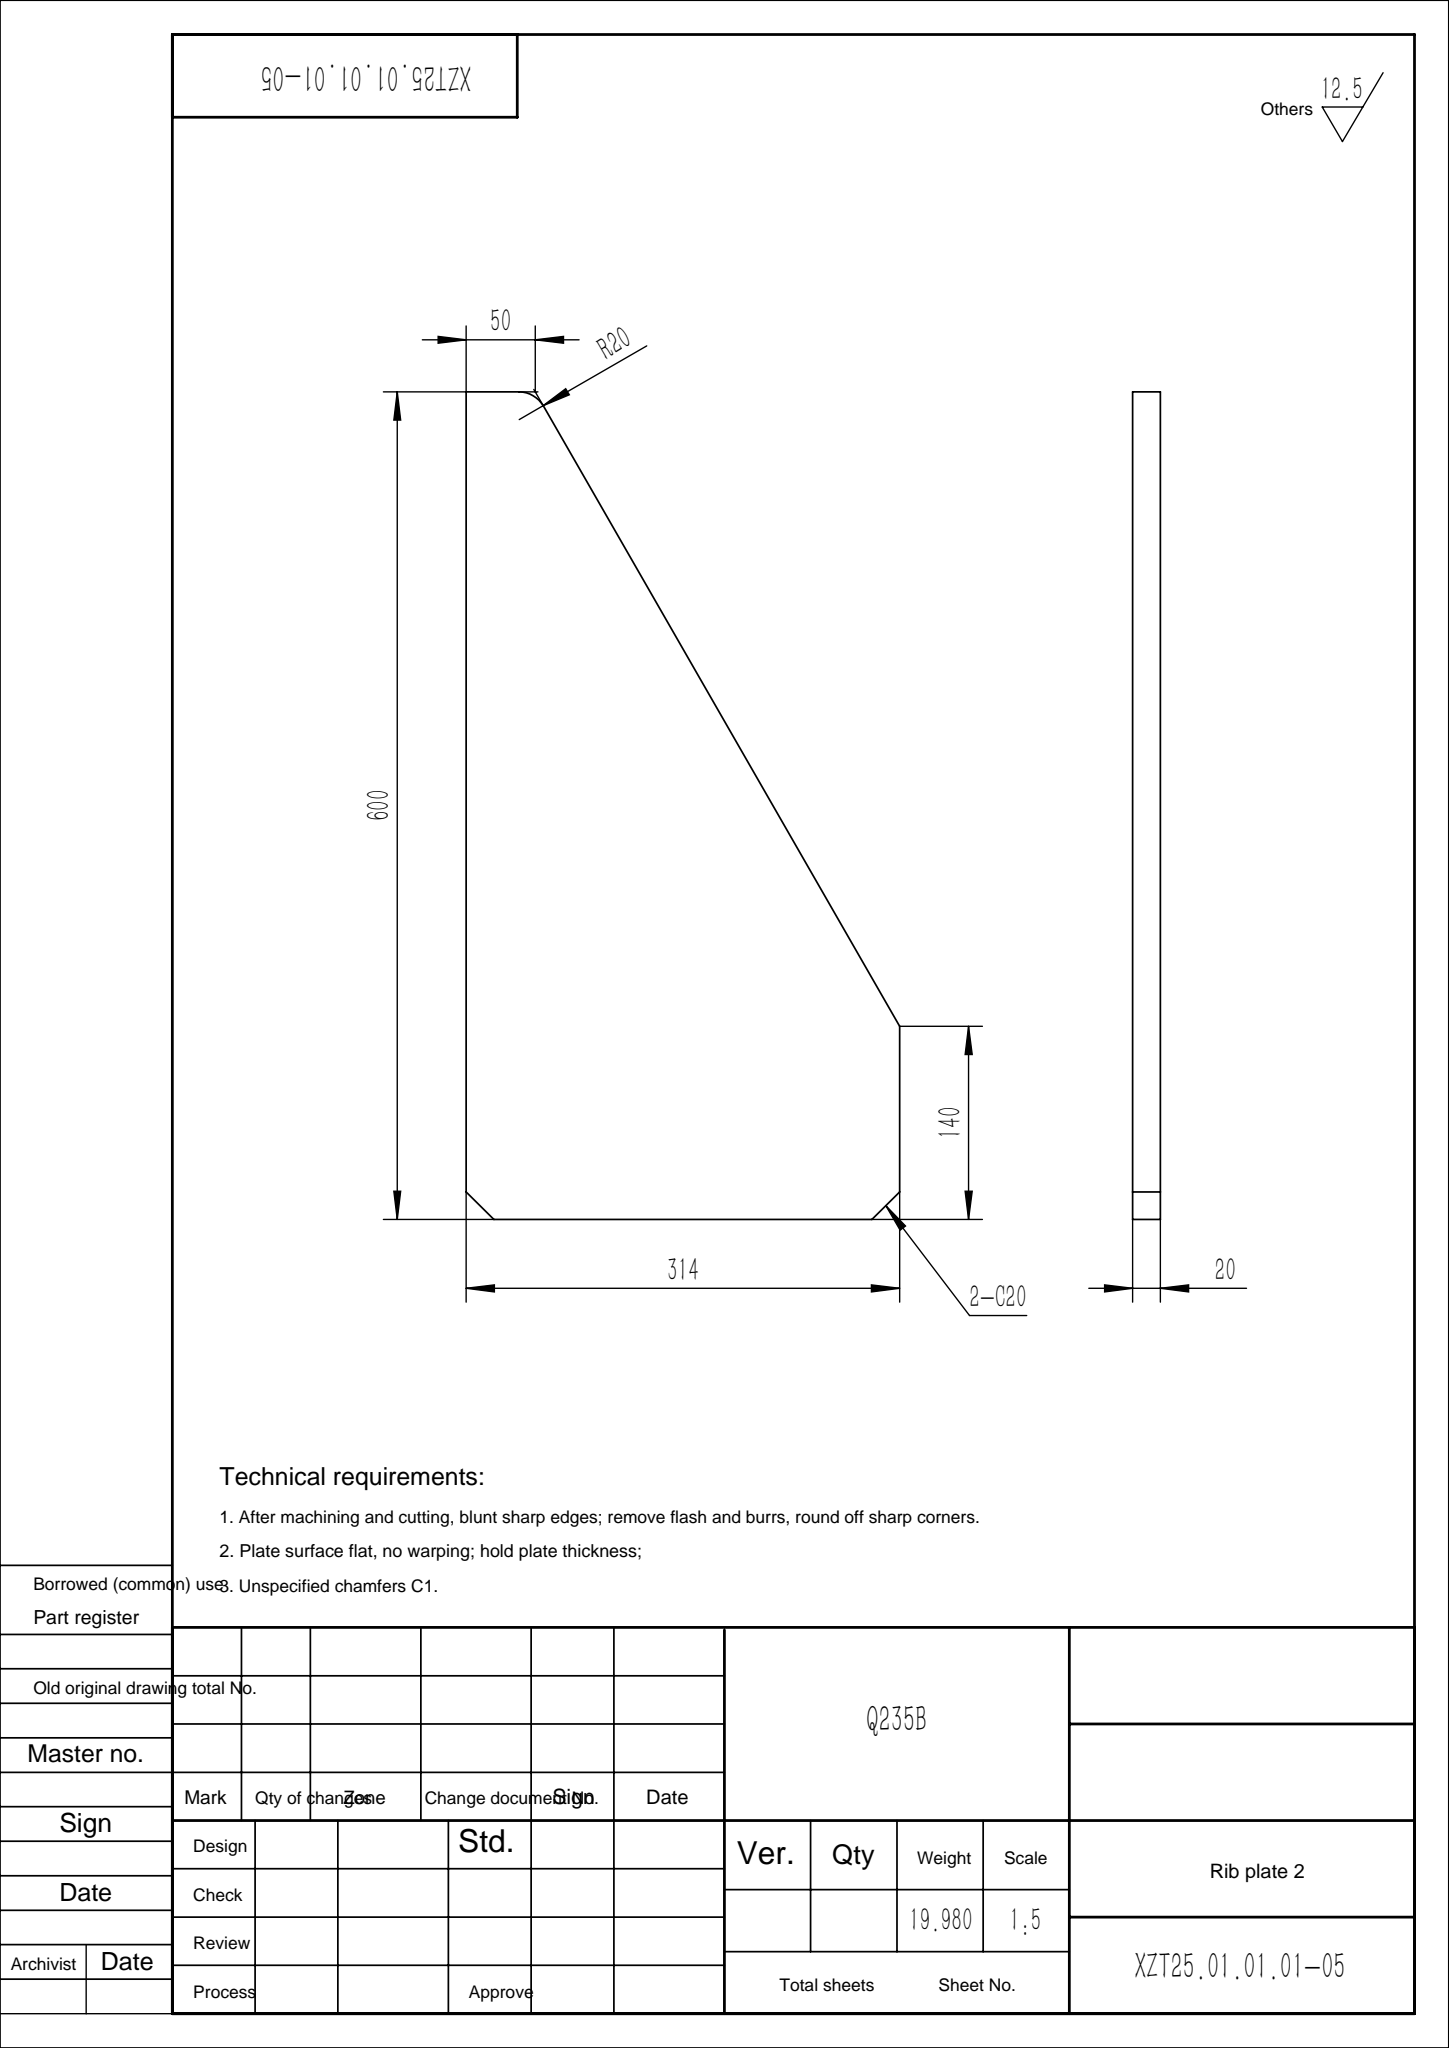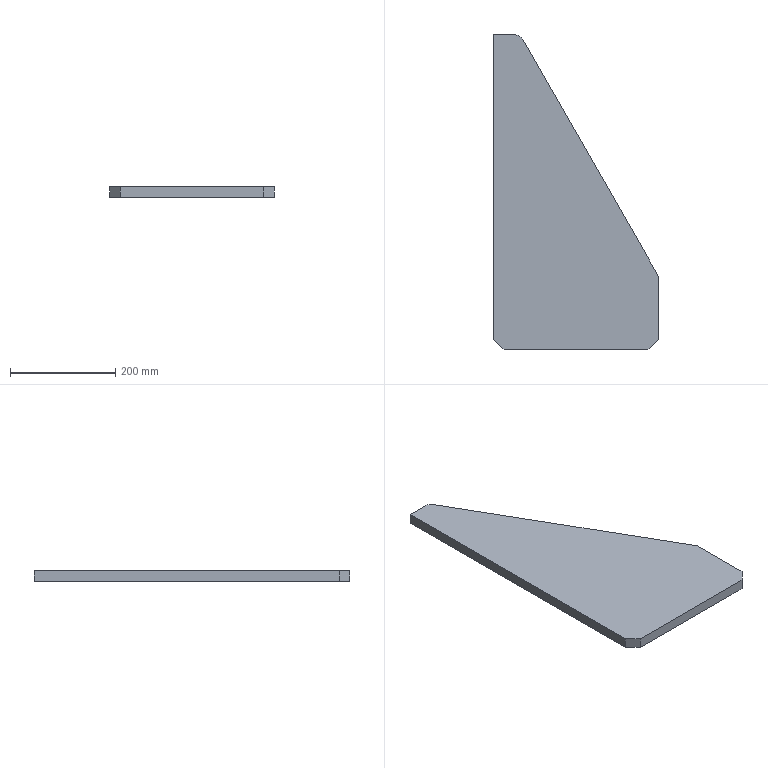Part | SolidWorks | features Chamfer 1, Extrusion 1, Fillet 1 | 1 solid | 10 faces | box 314 x 600 x 20 mm | volume 2545167 mm3 | plane 9 | cylinder 1 | commonest cylinder face diameters 40 x1
STEP:
#1=CARTESIAN_POINT('',(0.,600.,-10.));
#2=VERTEX_POINT('',#1);
#3=CARTESIAN_POINT('',(0.,20.,-10.));
#4=VERTEX_POINT('',#3);
#5=CARTESIAN_POINT('',(0.,600.,-10.));
#6=DIRECTION('',(0.,-1.,0.));
#7=VECTOR('',#6,1000.);
#8=LINE('',#5,#7);
#9=EDGE_CURVE('',#2,#4,#8,.T.);
#10=ORIENTED_EDGE('',*,*,#9,.T.);
#11=CARTESIAN_POINT('',(0.,20.,10.));
#12=VERTEX_POINT('',#11);
#13=CARTESIAN_POINT('',(0.,20.,10.));
#14=DIRECTION('',(0.,0.,1.));
#15=VECTOR('',#14,1000.);
#16=LINE('',#13,#15);
#17=EDGE_CURVE('',#4,#12,#16,.T.);
#18=ORIENTED_EDGE('',*,*,#17,.T.);
#19=CARTESIAN_POINT('',(0.,600.,10.));
#20=VERTEX_POINT('',#19);
#21=CARTESIAN_POINT('',(0.,600.,10.));
#22=DIRECTION('',(0.,-1.,0.));
#23=VECTOR('',#22,1000.);
#24=LINE('',#21,#23);
#25=EDGE_CURVE('',#20,#12,#24,.T.);
#26=ORIENTED_EDGE('',*,*,#25,.F.);
#27=CARTESIAN_POINT('',(0.,600.,10.));
#28=DIRECTION('',(0.,0.,-1.));
#29=VECTOR('',#28,1000.);
#30=LINE('',#27,#29);
#31=EDGE_CURVE('',#20,#2,#30,.T.);
#32=ORIENTED_EDGE('',*,*,#31,.T.);
#33=EDGE_LOOP('',(#10,#18,#26,#32));
#34=FACE_OUTER_BOUND('',#33,.T.);
#35=CARTESIAN_POINT('',(0.,600.,10.));
#36=DIRECTION('',(1.,0.,0.));
#37=DIRECTION('',(0.,1.,0.));
#38=AXIS2_PLACEMENT_3D('',#35,#36,#37);
#39=PLANE('',#38);
#40=ADVANCED_FACE('',(#34),#39,.F.);
#41=CARTESIAN_POINT('',(20.,0.,-10.));
#42=VERTEX_POINT('',#41);
#43=CARTESIAN_POINT('',(294.,0.,-10.));
#44=VERTEX_POINT('',#43);
#45=CARTESIAN_POINT('',(0.,0.,-10.));
#46=DIRECTION('',(1.,0.,0.));
#47=VECTOR('',#46,1000.);
#48=LINE('',#45,#47);
#49=EDGE_CURVE('',#42,#44,#48,.T.);
#50=ORIENTED_EDGE('',*,*,#49,.T.);
#51=CARTESIAN_POINT('',(294.,0.,10.));
#52=VERTEX_POINT('',#51);
#53=CARTESIAN_POINT('',(294.,0.,10.));
#54=DIRECTION('',(0.,0.,1.));
#55=VECTOR('',#54,1000.);
#56=LINE('',#53,#55);
#57=EDGE_CURVE('',#44,#52,#56,.T.);
#58=ORIENTED_EDGE('',*,*,#57,.T.);
#59=CARTESIAN_POINT('',(20.,0.,10.));
#60=VERTEX_POINT('',#59);
#61=CARTESIAN_POINT('',(0.,0.,10.));
#62=DIRECTION('',(1.,0.,0.));
#63=VECTOR('',#62,1000.);
#64=LINE('',#61,#63);
#65=EDGE_CURVE('',#60,#52,#64,.T.);
#66=ORIENTED_EDGE('',*,*,#65,.F.);
#67=CARTESIAN_POINT('',(20.,0.,10.));
#68=DIRECTION('',(0.,0.,-1.));
#69=VECTOR('',#68,1000.);
#70=LINE('',#67,#69);
#71=EDGE_CURVE('',#60,#42,#70,.T.);
#72=ORIENTED_EDGE('',*,*,#71,.T.);
#73=EDGE_LOOP('',(#50,#58,#66,#72));
#74=FACE_OUTER_BOUND('',#73,.T.);
#75=CARTESIAN_POINT('',(0.,0.,10.));
#76=DIRECTION('',(0.,1.,0.));
#77=DIRECTION('',(0.,0.,1.));
#78=AXIS2_PLACEMENT_3D('',#75,#76,#77);
#79=PLANE('',#78);
#80=ADVANCED_FACE('',(#74),#79,.F.);
#81=CARTESIAN_POINT('',(314.,20.,10.));
#82=VERTEX_POINT('',#81);
#83=CARTESIAN_POINT('',(314.,140.,10.));
#84=VERTEX_POINT('',#83);
#85=CARTESIAN_POINT('',(314.,0.,10.));
#86=DIRECTION('',(0.,1.,0.));
#87=VECTOR('',#86,1000.);
#88=LINE('',#85,#87);
#89=EDGE_CURVE('',#82,#84,#88,.T.);
#90=ORIENTED_EDGE('',*,*,#89,.F.);
#91=CARTESIAN_POINT('',(314.,20.,-10.));
#92=VERTEX_POINT('',#91);
#93=CARTESIAN_POINT('',(314.,20.,10.));
#94=DIRECTION('',(0.,0.,-1.));
#95=VECTOR('',#94,1000.);
#96=LINE('',#93,#95);
#97=EDGE_CURVE('',#82,#92,#96,.T.);
#98=ORIENTED_EDGE('',*,*,#97,.T.);
#99=CARTESIAN_POINT('',(314.,140.,-10.));
#100=VERTEX_POINT('',#99);
#101=CARTESIAN_POINT('',(314.,0.,-10.));
#102=DIRECTION('',(0.,1.,0.));
#103=VECTOR('',#102,1000.);
#104=LINE('',#101,#103);
#105=EDGE_CURVE('',#92,#100,#104,.T.);
#106=ORIENTED_EDGE('',*,*,#105,.T.);
#107=CARTESIAN_POINT('',(314.,140.,10.));
#108=DIRECTION('',(0.,0.,-1.));
#109=VECTOR('',#108,1000.);
#110=LINE('',#107,#109);
#111=EDGE_CURVE('',#84,#100,#110,.T.);
#112=ORIENTED_EDGE('',*,*,#111,.F.);
#113=EDGE_LOOP('',(#90,#98,#106,#112));
#114=FACE_OUTER_BOUND('',#113,.T.);
#115=CARTESIAN_POINT('',(314.,0.,10.));
#116=DIRECTION('',(-1.,0.,0.));
#117=DIRECTION('',(0.,0.,1.));
#118=AXIS2_PLACEMENT_3D('',#115,#116,#117);
#119=PLANE('',#118);
#120=ADVANCED_FACE('',(#114),#119,.F.);
#121=CARTESIAN_POINT('',(55.765,589.955,-10.));
#122=VERTEX_POINT('',#121);
#123=CARTESIAN_POINT('',(314.,140.,-10.));
#124=DIRECTION('',(-0.4978,0.8673,0.));
#125=VECTOR('',#124,1000.);
#126=LINE('',#123,#125);
#127=EDGE_CURVE('',#100,#122,#126,.T.);
#128=ORIENTED_EDGE('',*,*,#127,.T.);
#129=CARTESIAN_POINT('',(55.765,589.955,10.));
#130=VERTEX_POINT('',#129);
#131=CARTESIAN_POINT('',(55.765,589.955,10.));
#132=DIRECTION('',(0.,0.,1.));
#133=VECTOR('',#132,1000.);
#134=LINE('',#131,#133);
#135=EDGE_CURVE('',#122,#130,#134,.T.);
#136=ORIENTED_EDGE('',*,*,#135,.T.);
#137=CARTESIAN_POINT('',(314.,140.,10.));
#138=DIRECTION('',(-0.4978,0.8673,0.));
#139=VECTOR('',#138,1000.);
#140=LINE('',#137,#139);
#141=EDGE_CURVE('',#84,#130,#140,.T.);
#142=ORIENTED_EDGE('',*,*,#141,.F.);
#143=ORIENTED_EDGE('',*,*,#111,.T.);
#144=EDGE_LOOP('',(#128,#136,#142,#143));
#145=FACE_OUTER_BOUND('',#144,.T.);
#146=CARTESIAN_POINT('',(314.,140.,10.));
#147=DIRECTION('',(-0.8673,-0.4978,0.));
#148=DIRECTION('',(0.4978,-0.8673,0.));
#149=AXIS2_PLACEMENT_3D('',#146,#147,#148);
#150=PLANE('',#149);
#151=ADVANCED_FACE('',(#145),#150,.F.);
#152=CARTESIAN_POINT('',(38.419,600.,10.));
#153=VERTEX_POINT('',#152);
#154=CARTESIAN_POINT('',(50.,600.,10.));
#155=DIRECTION('',(-1.,0.,0.));
#156=VECTOR('',#155,1000.);
#157=LINE('',#154,#156);
#158=EDGE_CURVE('',#153,#20,#157,.T.);
#159=ORIENTED_EDGE('',*,*,#158,.F.);
#160=CARTESIAN_POINT('',(38.419,600.,-10.));
#161=VERTEX_POINT('',#160);
#162=CARTESIAN_POINT('',(38.419,600.,10.));
#163=DIRECTION('',(0.,0.,-1.));
#164=VECTOR('',#163,1000.);
#165=LINE('',#162,#164);
#166=EDGE_CURVE('',#153,#161,#165,.T.);
#167=ORIENTED_EDGE('',*,*,#166,.T.);
#168=CARTESIAN_POINT('',(50.,600.,-10.));
#169=DIRECTION('',(-1.,0.,0.));
#170=VECTOR('',#169,1000.);
#171=LINE('',#168,#170);
#172=EDGE_CURVE('',#161,#2,#171,.T.);
#173=ORIENTED_EDGE('',*,*,#172,.T.);
#174=ORIENTED_EDGE('',*,*,#31,.F.);
#175=EDGE_LOOP('',(#159,#167,#173,#174));
#176=FACE_OUTER_BOUND('',#175,.T.);
#177=CARTESIAN_POINT('',(50.,600.,10.));
#178=DIRECTION('',(0.,-1.,0.));
#179=DIRECTION('',(0.,0.,-1.));
#180=AXIS2_PLACEMENT_3D('',#177,#178,#179);
#181=PLANE('',#180);
#182=ADVANCED_FACE('',(#176),#181,.F.);
#183=ORIENTED_EDGE('',*,*,#65,.T.);
#184=CARTESIAN_POINT('',(147.,-147.,10.));
#185=DIRECTION('',(0.7071,0.7071,0.));
#186=VECTOR('',#185,1000.);
#187=LINE('',#184,#186);
#188=EDGE_CURVE('',#52,#82,#187,.T.);
#189=ORIENTED_EDGE('',*,*,#188,.T.);
#190=ORIENTED_EDGE('',*,*,#89,.T.);
#191=ORIENTED_EDGE('',*,*,#141,.T.);
#192=CARTESIAN_POINT('',(38.419,580.,10.));
#193=DIRECTION('',(0.,0.,1.));
#194=DIRECTION('',(1.,0.,0.));
#195=AXIS2_PLACEMENT_3D('',#192,#193,#194);
#196=CIRCLE('',#195,20.);
#197=EDGE_CURVE('',#130,#153,#196,.T.);
#198=ORIENTED_EDGE('',*,*,#197,.T.);
#199=ORIENTED_EDGE('',*,*,#158,.T.);
#200=ORIENTED_EDGE('',*,*,#25,.T.);
#201=CARTESIAN_POINT('',(10.,10.,10.));
#202=DIRECTION('',(0.7071,-0.7071,0.));
#203=VECTOR('',#202,1000.);
#204=LINE('',#201,#203);
#205=EDGE_CURVE('',#12,#60,#204,.T.);
#206=ORIENTED_EDGE('',*,*,#205,.T.);
#207=EDGE_LOOP('',(#183,#189,#190,#191,#198,#199,#200,#206));
#208=FACE_OUTER_BOUND('',#207,.T.);
#209=CARTESIAN_POINT('',(0.,0.,10.));
#210=DIRECTION('',(0.,0.,1.));
#211=DIRECTION('',(1.,0.,0.));
#212=AXIS2_PLACEMENT_3D('',#209,#210,#211);
#213=PLANE('',#212);
#214=ADVANCED_FACE('',(#208),#213,.T.);
#215=ORIENTED_EDGE('',*,*,#105,.F.);
#216=CARTESIAN_POINT('',(314.,20.,-10.));
#217=DIRECTION('',(-0.7071,-0.7071,0.));
#218=VECTOR('',#217,1000.);
#219=LINE('',#216,#218);
#220=EDGE_CURVE('',#92,#44,#219,.T.);
#221=ORIENTED_EDGE('',*,*,#220,.T.);
#222=ORIENTED_EDGE('',*,*,#49,.F.);
#223=CARTESIAN_POINT('',(20.,0.,-10.));
#224=DIRECTION('',(-0.7071,0.7071,0.));
#225=VECTOR('',#224,1000.);
#226=LINE('',#223,#225);
#227=EDGE_CURVE('',#42,#4,#226,.T.);
#228=ORIENTED_EDGE('',*,*,#227,.T.);
#229=ORIENTED_EDGE('',*,*,#9,.F.);
#230=ORIENTED_EDGE('',*,*,#172,.F.);
#231=CARTESIAN_POINT('',(38.419,580.,-10.));
#232=DIRECTION('',(0.,0.,-1.));
#233=DIRECTION('',(1.,0.,0.));
#234=AXIS2_PLACEMENT_3D('',#231,#232,#233);
#235=CIRCLE('',#234,20.);
#236=EDGE_CURVE('',#161,#122,#235,.T.);
#237=ORIENTED_EDGE('',*,*,#236,.T.);
#238=ORIENTED_EDGE('',*,*,#127,.F.);
#239=EDGE_LOOP('',(#215,#221,#222,#228,#229,#230,#237,#238));
#240=FACE_OUTER_BOUND('',#239,.T.);
#241=CARTESIAN_POINT('',(0.,0.,-10.));
#242=DIRECTION('',(0.,0.,1.));
#243=DIRECTION('',(1.,0.,0.));
#244=AXIS2_PLACEMENT_3D('',#241,#242,#243);
#245=PLANE('',#244);
#246=ADVANCED_FACE('',(#240),#245,.F.);
#247=ORIENTED_EDGE('',*,*,#197,.F.);
#248=ORIENTED_EDGE('',*,*,#135,.F.);
#249=ORIENTED_EDGE('',*,*,#236,.F.);
#250=ORIENTED_EDGE('',*,*,#166,.F.);
#251=EDGE_LOOP('',(#247,#248,#249,#250));
#252=FACE_OUTER_BOUND('',#251,.T.);
#253=CARTESIAN_POINT('',(38.419,580.,10.));
#254=DIRECTION('',(0.,0.,-1.));
#255=DIRECTION('',(-1.,0.,0.));
#256=AXIS2_PLACEMENT_3D('',#253,#254,#255);
#257=CYLINDRICAL_SURFACE('',#256,20.);
#258=ADVANCED_FACE('',(#252),#257,.T.);
#259=ORIENTED_EDGE('',*,*,#188,.F.);
#260=ORIENTED_EDGE('',*,*,#57,.F.);
#261=ORIENTED_EDGE('',*,*,#220,.F.);
#262=ORIENTED_EDGE('',*,*,#97,.F.);
#263=EDGE_LOOP('',(#259,#260,#261,#262));
#264=FACE_OUTER_BOUND('',#263,.T.);
#265=CARTESIAN_POINT('',(314.,20.,10.));
#266=DIRECTION('',(-0.7071,0.7071,0.));
#267=DIRECTION('',(0.,0.,-1.));
#268=AXIS2_PLACEMENT_3D('',#265,#266,#267);
#269=PLANE('',#268);
#270=ADVANCED_FACE('',(#264),#269,.F.);
#271=ORIENTED_EDGE('',*,*,#205,.F.);
#272=ORIENTED_EDGE('',*,*,#17,.F.);
#273=ORIENTED_EDGE('',*,*,#227,.F.);
#274=ORIENTED_EDGE('',*,*,#71,.F.);
#275=EDGE_LOOP('',(#271,#272,#273,#274));
#276=FACE_OUTER_BOUND('',#275,.T.);
#277=CARTESIAN_POINT('',(20.,0.,10.));
#278=DIRECTION('',(0.7071,0.7071,0.));
#279=DIRECTION('',(0.,0.,-1.));
#280=AXIS2_PLACEMENT_3D('',#277,#278,#279);
#281=PLANE('',#280);
#282=ADVANCED_FACE('',(#276),#281,.F.);
#283=CLOSED_SHELL('',(#40,#80,#120,#151,#182,#214,#246,#258,#270,#282));
#284=MANIFOLD_SOLID_BREP('',#283);
#285=CARTESIAN_POINT('',(0.,0.,0.));
#286=DIRECTION('',(0.,0.,1.));
#287=DIRECTION('',(1.,0.,0.));
#288=AXIS2_PLACEMENT_3D('',#285,#286,#287);
#289=(LENGTH_UNIT()NAMED_UNIT(*)SI_UNIT(.MILLI.,.METRE.));
#290=UNCERTAINTY_MEASURE_WITH_UNIT(LENGTH_MEASURE(0.00001),#289,'','');
#291=(NAMED_UNIT(*)PLANE_ANGLE_UNIT()SI_UNIT($,.RADIAN.));
#292=(NAMED_UNIT(*)SI_UNIT($,.STERADIAN.)SOLID_ANGLE_UNIT());
#293=(GEOMETRIC_REPRESENTATION_CONTEXT(3)GLOBAL_UNCERTAINTY_ASSIGNED_CONTEXT((#290))GLOBAL_UNIT_ASSIGNED_CONTEXT((#289,#291,#292))REPRESENTATION_CONTEXT('',''));
#294=ADVANCED_BREP_SHAPE_REPRESENTATION('',(#284,#288),#293);